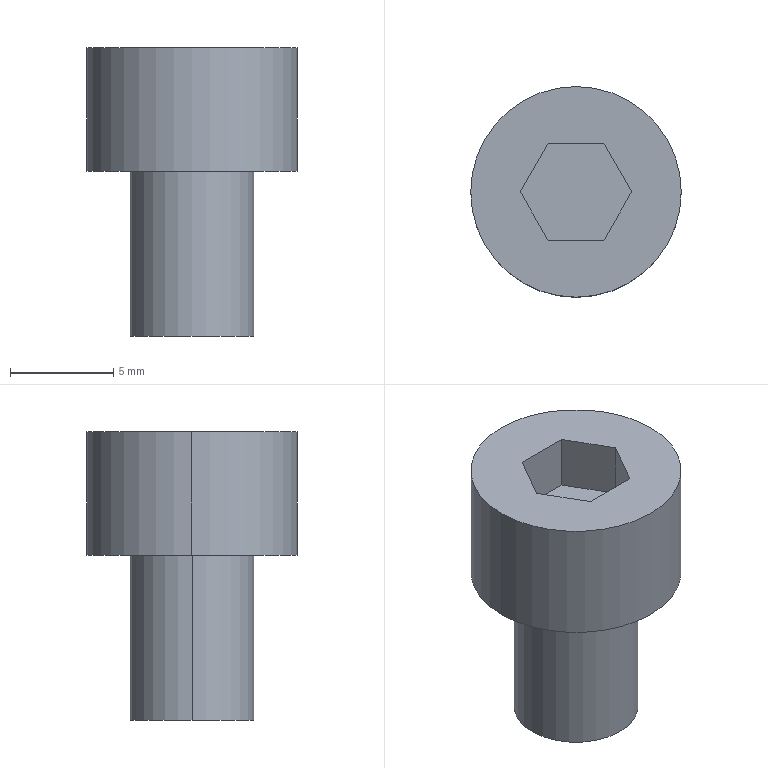Part | SolidWorks | features BaseBody 1 | 1 solid | 14 faces | box 10.2 x 10.2 x 14 mm | volume 665.334 mm3 | plane 10 | cylinder 4 | commonest cylinder face diameters 6 x2 10.2 x2
STEP:
#1=CARTESIAN_POINT('',(5.1,0.,0.));
#2=VERTEX_POINT('',#1);
#3=CARTESIAN_POINT('',(-5.1,0.,0.));
#4=VERTEX_POINT('',#3);
#5=CARTESIAN_POINT('',(0.,0.,0.));
#6=DIRECTION('',(0.,0.,1.));
#7=DIRECTION('',(1.,0.,0.));
#8=AXIS2_PLACEMENT_3D('',#5,#6,#7);
#9=CIRCLE('',#8,5.1);
#10=EDGE_CURVE('',#2,#4,#9,.T.);
#11=ORIENTED_EDGE('',*,*,#10,.T.);
#12=CARTESIAN_POINT('',(-5.1,0.,6.));
#13=VERTEX_POINT('',#12);
#14=CARTESIAN_POINT('',(-5.1,0.,0.));
#15=DIRECTION('',(0.,0.,1.));
#16=VECTOR('',#15,1000.);
#17=LINE('',#14,#16);
#18=EDGE_CURVE('',#4,#13,#17,.T.);
#19=ORIENTED_EDGE('',*,*,#18,.T.);
#20=CARTESIAN_POINT('',(5.1,0.,6.));
#21=VERTEX_POINT('',#20);
#22=CARTESIAN_POINT('',(0.,0.,6.));
#23=DIRECTION('',(0.,0.,-1.));
#24=DIRECTION('',(1.,0.,0.));
#25=AXIS2_PLACEMENT_3D('',#22,#23,#24);
#26=CIRCLE('',#25,5.1);
#27=EDGE_CURVE('',#13,#21,#26,.T.);
#28=ORIENTED_EDGE('',*,*,#27,.T.);
#29=CARTESIAN_POINT('',(5.1,0.,0.));
#30=DIRECTION('',(0.,0.,1.));
#31=VECTOR('',#30,1000.);
#32=LINE('',#29,#31);
#33=EDGE_CURVE('',#2,#21,#32,.T.);
#34=ORIENTED_EDGE('',*,*,#33,.F.);
#35=EDGE_LOOP('',(#11,#19,#28,#34));
#36=FACE_OUTER_BOUND('',#35,.T.);
#37=CARTESIAN_POINT('',(0.,0.,0.));
#38=DIRECTION('',(0.,0.,1.));
#39=DIRECTION('',(1.,0.,0.));
#40=AXIS2_PLACEMENT_3D('',#37,#38,#39);
#41=CYLINDRICAL_SURFACE('',#40,5.1);
#42=ADVANCED_FACE('',(#36),#41,.T.);
#43=CARTESIAN_POINT('',(3.,0.,-8.));
#44=VERTEX_POINT('',#43);
#45=CARTESIAN_POINT('',(-3.,0.,-8.));
#46=VERTEX_POINT('',#45);
#47=CARTESIAN_POINT('',(0.,0.,-8.));
#48=DIRECTION('',(0.,0.,1.));
#49=DIRECTION('',(1.,0.,0.));
#50=AXIS2_PLACEMENT_3D('',#47,#48,#49);
#51=CIRCLE('',#50,3.);
#52=EDGE_CURVE('',#44,#46,#51,.T.);
#53=ORIENTED_EDGE('',*,*,#52,.T.);
#54=CARTESIAN_POINT('',(-3.,0.,0.));
#55=VERTEX_POINT('',#54);
#56=CARTESIAN_POINT('',(-3.,0.,-8.));
#57=DIRECTION('',(0.,0.,1.));
#58=VECTOR('',#57,1000.);
#59=LINE('',#56,#58);
#60=EDGE_CURVE('',#46,#55,#59,.T.);
#61=ORIENTED_EDGE('',*,*,#60,.T.);
#62=CARTESIAN_POINT('',(3.,0.,0.));
#63=VERTEX_POINT('',#62);
#64=CARTESIAN_POINT('',(0.,0.,0.));
#65=DIRECTION('',(0.,0.,-1.));
#66=DIRECTION('',(1.,0.,0.));
#67=AXIS2_PLACEMENT_3D('',#64,#65,#66);
#68=CIRCLE('',#67,3.);
#69=EDGE_CURVE('',#55,#63,#68,.T.);
#70=ORIENTED_EDGE('',*,*,#69,.T.);
#71=CARTESIAN_POINT('',(3.,0.,-8.));
#72=DIRECTION('',(0.,0.,1.));
#73=VECTOR('',#72,1000.);
#74=LINE('',#71,#73);
#75=EDGE_CURVE('',#44,#63,#74,.T.);
#76=ORIENTED_EDGE('',*,*,#75,.F.);
#77=EDGE_LOOP('',(#53,#61,#70,#76));
#78=FACE_OUTER_BOUND('',#77,.T.);
#79=CARTESIAN_POINT('',(0.,0.,-8.));
#80=DIRECTION('',(0.,0.,1.));
#81=DIRECTION('',(1.,0.,0.));
#82=AXIS2_PLACEMENT_3D('',#79,#80,#81);
#83=CYLINDRICAL_SURFACE('',#82,3.);
#84=ADVANCED_FACE('',(#78),#83,.T.);
#85=ORIENTED_EDGE('',*,*,#18,.F.);
#86=CARTESIAN_POINT('',(0.,0.,0.));
#87=DIRECTION('',(0.,0.,1.));
#88=DIRECTION('',(1.,0.,0.));
#89=AXIS2_PLACEMENT_3D('',#86,#87,#88);
#90=CIRCLE('',#89,5.1);
#91=EDGE_CURVE('',#4,#2,#90,.T.);
#92=ORIENTED_EDGE('',*,*,#91,.T.);
#93=ORIENTED_EDGE('',*,*,#33,.T.);
#94=CARTESIAN_POINT('',(0.,0.,6.));
#95=DIRECTION('',(0.,0.,-1.));
#96=DIRECTION('',(1.,0.,0.));
#97=AXIS2_PLACEMENT_3D('',#94,#95,#96);
#98=CIRCLE('',#97,5.1);
#99=EDGE_CURVE('',#21,#13,#98,.T.);
#100=ORIENTED_EDGE('',*,*,#99,.T.);
#101=EDGE_LOOP('',(#85,#92,#93,#100));
#102=FACE_OUTER_BOUND('',#101,.T.);
#103=CARTESIAN_POINT('',(0.,0.,0.));
#104=DIRECTION('',(0.,0.,1.));
#105=DIRECTION('',(1.,0.,0.));
#106=AXIS2_PLACEMENT_3D('',#103,#104,#105);
#107=CYLINDRICAL_SURFACE('',#106,5.1);
#108=ADVANCED_FACE('',(#102),#107,.T.);
#109=CARTESIAN_POINT('',(0.,0.,0.));
#110=DIRECTION('',(0.,0.,-1.));
#111=DIRECTION('',(1.,0.,0.));
#112=AXIS2_PLACEMENT_3D('',#109,#110,#111);
#113=CIRCLE('',#112,3.);
#114=EDGE_CURVE('',#63,#55,#113,.T.);
#115=ORIENTED_EDGE('',*,*,#114,.F.);
#116=ORIENTED_EDGE('',*,*,#69,.F.);
#117=EDGE_LOOP('',(#115,#116));
#118=FACE_BOUND('',#117,.T.);
#119=ORIENTED_EDGE('',*,*,#10,.F.);
#120=ORIENTED_EDGE('',*,*,#91,.F.);
#121=EDGE_LOOP('',(#119,#120));
#122=FACE_OUTER_BOUND('',#121,.T.);
#123=CARTESIAN_POINT('',(0.,0.,0.));
#124=DIRECTION('',(0.,0.,1.));
#125=DIRECTION('',(1.,0.,0.));
#126=AXIS2_PLACEMENT_3D('',#123,#124,#125);
#127=PLANE('',#126);
#128=ADVANCED_FACE('',(#118,#122),#127,.F.);
#129=CARTESIAN_POINT('',(-1.35,-2.338,6.));
#130=VERTEX_POINT('',#129);
#131=CARTESIAN_POINT('',(-2.7,0.,6.));
#132=VERTEX_POINT('',#131);
#133=CARTESIAN_POINT('',(-1.35,-2.338,6.));
#134=DIRECTION('',(-0.5,0.866,0.));
#135=VECTOR('',#134,1000.);
#136=LINE('',#133,#135);
#137=EDGE_CURVE('',#130,#132,#136,.T.);
#138=ORIENTED_EDGE('',*,*,#137,.T.);
#139=CARTESIAN_POINT('',(-1.35,2.338,6.));
#140=VERTEX_POINT('',#139);
#141=CARTESIAN_POINT('',(-2.7,0.,6.));
#142=DIRECTION('',(0.5,0.866,0.));
#143=VECTOR('',#142,1000.);
#144=LINE('',#141,#143);
#145=EDGE_CURVE('',#132,#140,#144,.T.);
#146=ORIENTED_EDGE('',*,*,#145,.T.);
#147=CARTESIAN_POINT('',(1.35,2.338,6.));
#148=VERTEX_POINT('',#147);
#149=CARTESIAN_POINT('',(0.,2.338,6.));
#150=DIRECTION('',(1.,0.,0.));
#151=VECTOR('',#150,1000.);
#152=LINE('',#149,#151);
#153=EDGE_CURVE('',#140,#148,#152,.T.);
#154=ORIENTED_EDGE('',*,*,#153,.T.);
#155=CARTESIAN_POINT('',(2.7,0.,6.));
#156=VERTEX_POINT('',#155);
#157=CARTESIAN_POINT('',(1.35,2.338,6.));
#158=DIRECTION('',(0.5,-0.866,0.));
#159=VECTOR('',#158,1000.);
#160=LINE('',#157,#159);
#161=EDGE_CURVE('',#148,#156,#160,.T.);
#162=ORIENTED_EDGE('',*,*,#161,.T.);
#163=CARTESIAN_POINT('',(1.35,-2.338,6.));
#164=VERTEX_POINT('',#163);
#165=CARTESIAN_POINT('',(2.7,0.,6.));
#166=DIRECTION('',(-0.5,-0.866,0.));
#167=VECTOR('',#166,1000.);
#168=LINE('',#165,#167);
#169=EDGE_CURVE('',#156,#164,#168,.T.);
#170=ORIENTED_EDGE('',*,*,#169,.T.);
#171=CARTESIAN_POINT('',(0.,-2.338,6.));
#172=DIRECTION('',(-1.,0.,0.));
#173=VECTOR('',#172,1000.);
#174=LINE('',#171,#173);
#175=EDGE_CURVE('',#164,#130,#174,.T.);
#176=ORIENTED_EDGE('',*,*,#175,.T.);
#177=EDGE_LOOP('',(#138,#146,#154,#162,#170,#176));
#178=FACE_BOUND('',#177,.T.);
#179=ORIENTED_EDGE('',*,*,#99,.F.);
#180=ORIENTED_EDGE('',*,*,#27,.F.);
#181=EDGE_LOOP('',(#179,#180));
#182=FACE_OUTER_BOUND('',#181,.T.);
#183=CARTESIAN_POINT('',(0.,0.,6.));
#184=DIRECTION('',(0.,0.,1.));
#185=DIRECTION('',(1.,0.,0.));
#186=AXIS2_PLACEMENT_3D('',#183,#184,#185);
#187=PLANE('',#186);
#188=ADVANCED_FACE('',(#178,#182),#187,.T.);
#189=ORIENTED_EDGE('',*,*,#60,.F.);
#190=CARTESIAN_POINT('',(0.,0.,-8.));
#191=DIRECTION('',(0.,0.,1.));
#192=DIRECTION('',(1.,0.,0.));
#193=AXIS2_PLACEMENT_3D('',#190,#191,#192);
#194=CIRCLE('',#193,3.);
#195=EDGE_CURVE('',#46,#44,#194,.T.);
#196=ORIENTED_EDGE('',*,*,#195,.T.);
#197=ORIENTED_EDGE('',*,*,#75,.T.);
#198=ORIENTED_EDGE('',*,*,#114,.T.);
#199=EDGE_LOOP('',(#189,#196,#197,#198));
#200=FACE_OUTER_BOUND('',#199,.T.);
#201=CARTESIAN_POINT('',(0.,0.,-8.));
#202=DIRECTION('',(0.,0.,1.));
#203=DIRECTION('',(1.,0.,0.));
#204=AXIS2_PLACEMENT_3D('',#201,#202,#203);
#205=CYLINDRICAL_SURFACE('',#204,3.);
#206=ADVANCED_FACE('',(#200),#205,.T.);
#207=ORIENTED_EDGE('',*,*,#145,.F.);
#208=CARTESIAN_POINT('',(-2.7,0.,3.3));
#209=VERTEX_POINT('',#208);
#210=CARTESIAN_POINT('',(-2.7,0.,3.3));
#211=DIRECTION('',(0.,0.,-1.));
#212=VECTOR('',#211,1000.);
#213=LINE('',#210,#212);
#214=EDGE_CURVE('',#132,#209,#213,.T.);
#215=ORIENTED_EDGE('',*,*,#214,.T.);
#216=CARTESIAN_POINT('',(-1.35,2.338,3.3));
#217=VERTEX_POINT('',#216);
#218=CARTESIAN_POINT('',(-1.35,2.338,3.3));
#219=DIRECTION('',(0.5,0.866,0.));
#220=VECTOR('',#219,1000.);
#221=LINE('',#218,#220);
#222=EDGE_CURVE('',#209,#217,#221,.T.);
#223=ORIENTED_EDGE('',*,*,#222,.T.);
#224=CARTESIAN_POINT('',(-1.35,2.338,3.3));
#225=DIRECTION('',(0.,0.,1.));
#226=VECTOR('',#225,1000.);
#227=LINE('',#224,#226);
#228=EDGE_CURVE('',#217,#140,#227,.T.);
#229=ORIENTED_EDGE('',*,*,#228,.T.);
#230=EDGE_LOOP('',(#207,#215,#223,#229));
#231=FACE_OUTER_BOUND('',#230,.T.);
#232=CARTESIAN_POINT('',(-1.35,2.338,3.3));
#233=DIRECTION('',(0.866,-0.5,0.));
#234=DIRECTION('',(0.5,0.866,0.));
#235=AXIS2_PLACEMENT_3D('',#232,#233,#234);
#236=PLANE('',#235);
#237=ADVANCED_FACE('',(#231),#236,.T.);
#238=ORIENTED_EDGE('',*,*,#137,.F.);
#239=CARTESIAN_POINT('',(-1.35,-2.338,3.3));
#240=VERTEX_POINT('',#239);
#241=CARTESIAN_POINT('',(-1.35,-2.338,3.3));
#242=DIRECTION('',(0.,0.,-1.));
#243=VECTOR('',#242,1000.);
#244=LINE('',#241,#243);
#245=EDGE_CURVE('',#130,#240,#244,.T.);
#246=ORIENTED_EDGE('',*,*,#245,.T.);
#247=CARTESIAN_POINT('',(-2.7,0.,3.3));
#248=DIRECTION('',(-0.5,0.866,0.));
#249=VECTOR('',#248,1000.);
#250=LINE('',#247,#249);
#251=EDGE_CURVE('',#240,#209,#250,.T.);
#252=ORIENTED_EDGE('',*,*,#251,.T.);
#253=ORIENTED_EDGE('',*,*,#214,.F.);
#254=EDGE_LOOP('',(#238,#246,#252,#253));
#255=FACE_OUTER_BOUND('',#254,.T.);
#256=CARTESIAN_POINT('',(-2.7,0.,3.3));
#257=DIRECTION('',(0.866,0.5,0.));
#258=DIRECTION('',(-0.5,0.866,0.));
#259=AXIS2_PLACEMENT_3D('',#256,#257,#258);
#260=PLANE('',#259);
#261=ADVANCED_FACE('',(#255),#260,.T.);
#262=ORIENTED_EDGE('',*,*,#175,.F.);
#263=CARTESIAN_POINT('',(1.35,-2.338,3.3));
#264=VERTEX_POINT('',#263);
#265=CARTESIAN_POINT('',(1.35,-2.338,3.3));
#266=DIRECTION('',(0.,0.,-1.));
#267=VECTOR('',#266,1000.);
#268=LINE('',#265,#267);
#269=EDGE_CURVE('',#164,#264,#268,.T.);
#270=ORIENTED_EDGE('',*,*,#269,.T.);
#271=CARTESIAN_POINT('',(-1.35,-2.338,3.3));
#272=DIRECTION('',(-1.,0.,0.));
#273=VECTOR('',#272,1000.);
#274=LINE('',#271,#273);
#275=EDGE_CURVE('',#264,#240,#274,.T.);
#276=ORIENTED_EDGE('',*,*,#275,.T.);
#277=ORIENTED_EDGE('',*,*,#245,.F.);
#278=EDGE_LOOP('',(#262,#270,#276,#277));
#279=FACE_OUTER_BOUND('',#278,.T.);
#280=CARTESIAN_POINT('',(-1.35,-2.338,3.3));
#281=DIRECTION('',(0.,1.,0.));
#282=DIRECTION('',(-1.,0.,0.));
#283=AXIS2_PLACEMENT_3D('',#280,#281,#282);
#284=PLANE('',#283);
#285=ADVANCED_FACE('',(#279),#284,.T.);
#286=ORIENTED_EDGE('',*,*,#169,.F.);
#287=CARTESIAN_POINT('',(2.7,0.,3.3));
#288=VERTEX_POINT('',#287);
#289=CARTESIAN_POINT('',(2.7,0.,3.3));
#290=DIRECTION('',(0.,0.,-1.));
#291=VECTOR('',#290,1000.);
#292=LINE('',#289,#291);
#293=EDGE_CURVE('',#156,#288,#292,.T.);
#294=ORIENTED_EDGE('',*,*,#293,.T.);
#295=CARTESIAN_POINT('',(1.35,-2.338,3.3));
#296=DIRECTION('',(-0.5,-0.866,0.));
#297=VECTOR('',#296,1000.);
#298=LINE('',#295,#297);
#299=EDGE_CURVE('',#288,#264,#298,.T.);
#300=ORIENTED_EDGE('',*,*,#299,.T.);
#301=ORIENTED_EDGE('',*,*,#269,.F.);
#302=EDGE_LOOP('',(#286,#294,#300,#301));
#303=FACE_OUTER_BOUND('',#302,.T.);
#304=CARTESIAN_POINT('',(1.35,-2.338,3.3));
#305=DIRECTION('',(-0.866,0.5,0.));
#306=DIRECTION('',(-0.5,-0.866,0.));
#307=AXIS2_PLACEMENT_3D('',#304,#305,#306);
#308=PLANE('',#307);
#309=ADVANCED_FACE('',(#303),#308,.T.);
#310=ORIENTED_EDGE('',*,*,#161,.F.);
#311=CARTESIAN_POINT('',(1.35,2.338,3.3));
#312=VERTEX_POINT('',#311);
#313=CARTESIAN_POINT('',(1.35,2.338,3.3));
#314=DIRECTION('',(0.,0.,-1.));
#315=VECTOR('',#314,1000.);
#316=LINE('',#313,#315);
#317=EDGE_CURVE('',#148,#312,#316,.T.);
#318=ORIENTED_EDGE('',*,*,#317,.T.);
#319=CARTESIAN_POINT('',(2.7,0.,3.3));
#320=DIRECTION('',(0.5,-0.866,0.));
#321=VECTOR('',#320,1000.);
#322=LINE('',#319,#321);
#323=EDGE_CURVE('',#312,#288,#322,.T.);
#324=ORIENTED_EDGE('',*,*,#323,.T.);
#325=ORIENTED_EDGE('',*,*,#293,.F.);
#326=EDGE_LOOP('',(#310,#318,#324,#325));
#327=FACE_OUTER_BOUND('',#326,.T.);
#328=CARTESIAN_POINT('',(2.7,0.,3.3));
#329=DIRECTION('',(-0.866,-0.5,0.));
#330=DIRECTION('',(0.5,-0.866,0.));
#331=AXIS2_PLACEMENT_3D('',#328,#329,#330);
#332=PLANE('',#331);
#333=ADVANCED_FACE('',(#327),#332,.T.);
#334=ORIENTED_EDGE('',*,*,#153,.F.);
#335=ORIENTED_EDGE('',*,*,#228,.F.);
#336=CARTESIAN_POINT('',(1.35,2.338,3.3));
#337=DIRECTION('',(1.,0.,0.));
#338=VECTOR('',#337,1000.);
#339=LINE('',#336,#338);
#340=EDGE_CURVE('',#217,#312,#339,.T.);
#341=ORIENTED_EDGE('',*,*,#340,.T.);
#342=ORIENTED_EDGE('',*,*,#317,.F.);
#343=EDGE_LOOP('',(#334,#335,#341,#342));
#344=FACE_OUTER_BOUND('',#343,.T.);
#345=CARTESIAN_POINT('',(1.35,2.338,3.3));
#346=DIRECTION('',(0.,-1.,0.));
#347=DIRECTION('',(0.,0.,-1.));
#348=AXIS2_PLACEMENT_3D('',#345,#346,#347);
#349=PLANE('',#348);
#350=ADVANCED_FACE('',(#344),#349,.T.);
#351=ORIENTED_EDGE('',*,*,#52,.F.);
#352=ORIENTED_EDGE('',*,*,#195,.F.);
#353=EDGE_LOOP('',(#351,#352));
#354=FACE_OUTER_BOUND('',#353,.T.);
#355=CARTESIAN_POINT('',(0.,0.,-8.));
#356=DIRECTION('',(0.,0.,1.));
#357=DIRECTION('',(1.,0.,0.));
#358=AXIS2_PLACEMENT_3D('',#355,#356,#357);
#359=PLANE('',#358);
#360=ADVANCED_FACE('',(#354),#359,.F.);
#361=ORIENTED_EDGE('',*,*,#275,.F.);
#362=ORIENTED_EDGE('',*,*,#299,.F.);
#363=ORIENTED_EDGE('',*,*,#323,.F.);
#364=ORIENTED_EDGE('',*,*,#340,.F.);
#365=ORIENTED_EDGE('',*,*,#222,.F.);
#366=ORIENTED_EDGE('',*,*,#251,.F.);
#367=EDGE_LOOP('',(#361,#362,#363,#364,#365,#366));
#368=FACE_OUTER_BOUND('',#367,.T.);
#369=CARTESIAN_POINT('',(0.,0.,3.3));
#370=DIRECTION('',(0.,0.,1.));
#371=DIRECTION('',(1.,0.,0.));
#372=AXIS2_PLACEMENT_3D('',#369,#370,#371);
#373=PLANE('',#372);
#374=ADVANCED_FACE('',(#368),#373,.T.);
#375=CLOSED_SHELL('',(#42,#84,#108,#128,#188,#206,#237,#261,#285,#309,#333,#350,#360,#374));
#376=MANIFOLD_SOLID_BREP('',#375);
#377=CARTESIAN_POINT('',(0.,0.,0.));
#378=DIRECTION('',(0.,0.,1.));
#379=DIRECTION('',(1.,0.,0.));
#380=AXIS2_PLACEMENT_3D('',#377,#378,#379);
#381=(LENGTH_UNIT()NAMED_UNIT(*)SI_UNIT(.MILLI.,.METRE.));
#382=UNCERTAINTY_MEASURE_WITH_UNIT(LENGTH_MEASURE(0.00001),#381,'','');
#383=(NAMED_UNIT(*)PLANE_ANGLE_UNIT()SI_UNIT($,.RADIAN.));
#384=(NAMED_UNIT(*)SI_UNIT($,.STERADIAN.)SOLID_ANGLE_UNIT());
#385=(GEOMETRIC_REPRESENTATION_CONTEXT(3)GLOBAL_UNCERTAINTY_ASSIGNED_CONTEXT((#382))GLOBAL_UNIT_ASSIGNED_CONTEXT((#381,#383,#384))REPRESENTATION_CONTEXT('',''));
#386=ADVANCED_BREP_SHAPE_REPRESENTATION('',(#376,#380),#385);